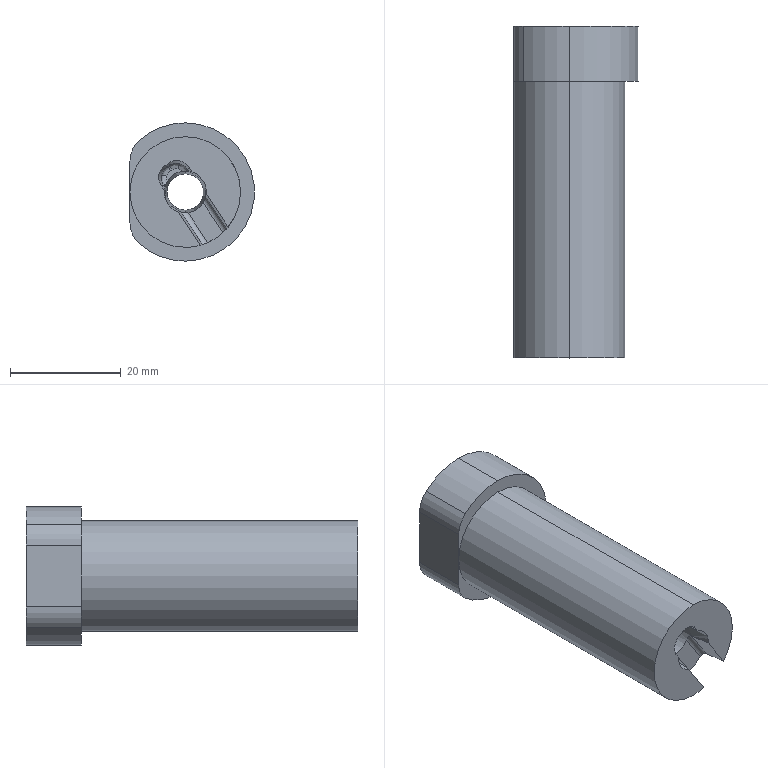Part | STEP file | 1 solid | 31 faces | box 22.5 x 60 x 25 mm | volume 17728 mm3 | cylinder 14 | plane 11 | spline 4 | cone 2 | commonest cylinder face diameters 2 x5 25 x3 5 x2 10 x2 20 x2